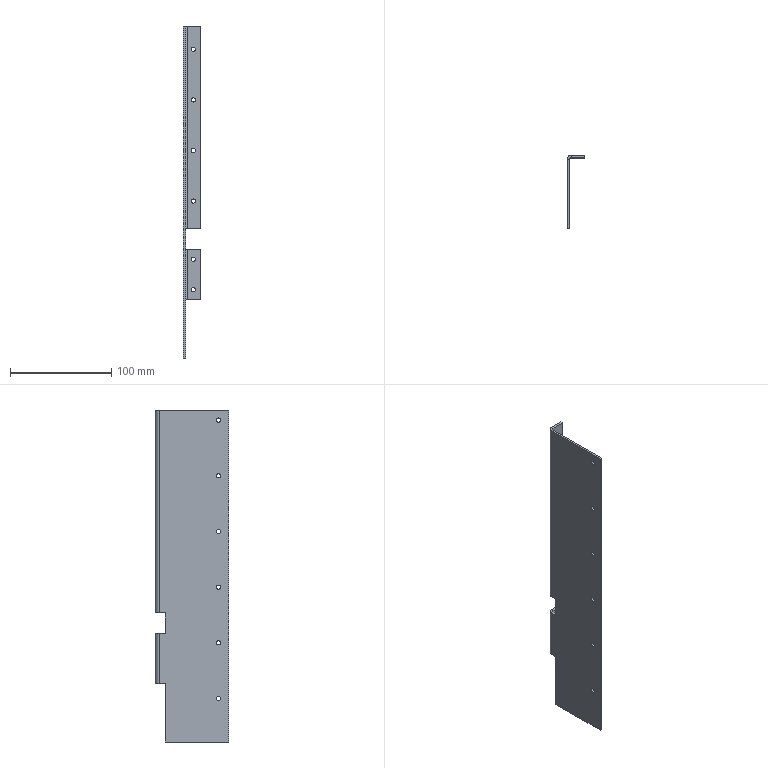Part | STEP file | 64605551 | 1 solid | 52 faces | box 17.5 x 72.5 x 328 mm | volume 65751 mm3 | cylinder 28 | plane 24 | commonest cylinder face diameters 4.2 x24 3 x2 8 x2